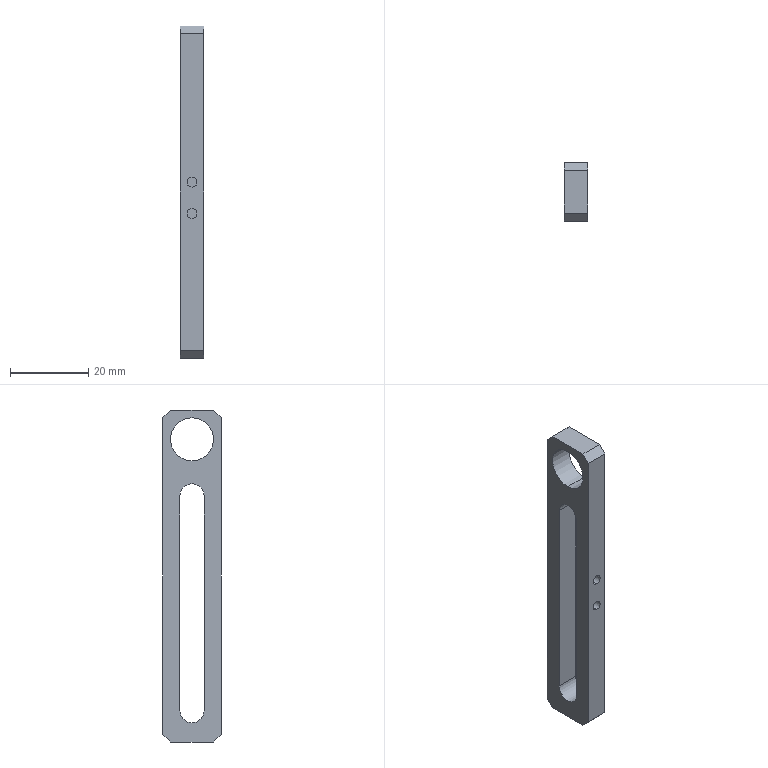Part | SolidWorks | features HoleWzd 2, Chamfer 1, Extrusion 1 | 1 solid | 21 faces | box 6 x 15 x 85 mm | volume 4761 mm3 | plane 12 | cylinder 9 | commonest cylinder face diameters 2.5 x4 6.2 x3 11 x2
STEP:
#1=CARTESIAN_POINT('',(3.,-10.6,-41.25));
#2=VERTEX_POINT('',#1);
#3=CARTESIAN_POINT('',(3.,-10.6,-38.75));
#4=VERTEX_POINT('',#3);
#5=CARTESIAN_POINT('',(3.,-10.6,-40.));
#6=DIRECTION('',(0.,1.,0.));
#7=DIRECTION('',(0.,0.,1.));
#8=AXIS2_PLACEMENT_3D('',#5,#6,#7);
#9=CIRCLE('',#8,1.25);
#10=EDGE_CURVE('',#2,#4,#9,.T.);
#11=ORIENTED_EDGE('',*,*,#10,.T.);
#12=CARTESIAN_POINT('',(3.,-15.,-38.75));
#13=VERTEX_POINT('',#12);
#14=CARTESIAN_POINT('',(3.,-15.,-38.75));
#15=DIRECTION('',(0.,-1.,0.));
#16=VECTOR('',#15,1000.);
#17=LINE('',#14,#16);
#18=EDGE_CURVE('',#4,#13,#17,.T.);
#19=ORIENTED_EDGE('',*,*,#18,.T.);
#20=CARTESIAN_POINT('',(3.,-15.,-41.25));
#21=VERTEX_POINT('',#20);
#22=CARTESIAN_POINT('',(3.,-15.,-40.));
#23=DIRECTION('',(0.,-1.,0.));
#24=DIRECTION('',(0.,0.,-1.));
#25=AXIS2_PLACEMENT_3D('',#22,#23,#24);
#26=CIRCLE('',#25,1.25);
#27=EDGE_CURVE('',#13,#21,#26,.T.);
#28=ORIENTED_EDGE('',*,*,#27,.T.);
#29=CARTESIAN_POINT('',(3.,-15.,-41.25));
#30=DIRECTION('',(0.,-1.,0.));
#31=VECTOR('',#30,1000.);
#32=LINE('',#29,#31);
#33=EDGE_CURVE('',#2,#21,#32,.T.);
#34=ORIENTED_EDGE('',*,*,#33,.F.);
#35=EDGE_LOOP('',(#11,#19,#28,#34));
#36=FACE_OUTER_BOUND('',#35,.T.);
#37=CARTESIAN_POINT('',(3.,-15.,-40.));
#38=DIRECTION('',(0.,-1.,0.));
#39=DIRECTION('',(0.,0.,-1.));
#40=AXIS2_PLACEMENT_3D('',#37,#38,#39);
#41=CYLINDRICAL_SURFACE('',#40,1.25);
#42=ADVANCED_FACE('',(#36),#41,.F.);
#43=CARTESIAN_POINT('',(3.,-10.6,-49.25));
#44=VERTEX_POINT('',#43);
#45=CARTESIAN_POINT('',(3.,-10.6,-46.75));
#46=VERTEX_POINT('',#45);
#47=CARTESIAN_POINT('',(3.,-10.6,-48.));
#48=DIRECTION('',(0.,1.,0.));
#49=DIRECTION('',(0.,0.,1.));
#50=AXIS2_PLACEMENT_3D('',#47,#48,#49);
#51=CIRCLE('',#50,1.25);
#52=EDGE_CURVE('',#44,#46,#51,.T.);
#53=ORIENTED_EDGE('',*,*,#52,.T.);
#54=CARTESIAN_POINT('',(3.,-15.,-46.75));
#55=VERTEX_POINT('',#54);
#56=CARTESIAN_POINT('',(3.,-15.,-46.75));
#57=DIRECTION('',(0.,-1.,0.));
#58=VECTOR('',#57,1000.);
#59=LINE('',#56,#58);
#60=EDGE_CURVE('',#46,#55,#59,.T.);
#61=ORIENTED_EDGE('',*,*,#60,.T.);
#62=CARTESIAN_POINT('',(3.,-15.,-49.25));
#63=VERTEX_POINT('',#62);
#64=CARTESIAN_POINT('',(3.,-15.,-48.));
#65=DIRECTION('',(0.,-1.,0.));
#66=DIRECTION('',(0.,0.,-1.));
#67=AXIS2_PLACEMENT_3D('',#64,#65,#66);
#68=CIRCLE('',#67,1.25);
#69=EDGE_CURVE('',#55,#63,#68,.T.);
#70=ORIENTED_EDGE('',*,*,#69,.T.);
#71=CARTESIAN_POINT('',(3.,-15.,-49.25));
#72=DIRECTION('',(0.,-1.,0.));
#73=VECTOR('',#72,1000.);
#74=LINE('',#71,#73);
#75=EDGE_CURVE('',#44,#63,#74,.T.);
#76=ORIENTED_EDGE('',*,*,#75,.F.);
#77=EDGE_LOOP('',(#53,#61,#70,#76));
#78=FACE_OUTER_BOUND('',#77,.T.);
#79=CARTESIAN_POINT('',(3.,-15.,-48.));
#80=DIRECTION('',(0.,-1.,0.));
#81=DIRECTION('',(0.,0.,-1.));
#82=AXIS2_PLACEMENT_3D('',#79,#80,#81);
#83=CYLINDRICAL_SURFACE('',#82,1.25);
#84=ADVANCED_FACE('',(#78),#83,.F.);
#85=CARTESIAN_POINT('',(0.,-7.5,-2.));
#86=VERTEX_POINT('',#85);
#87=CARTESIAN_POINT('',(0.,-7.5,-13.));
#88=VERTEX_POINT('',#87);
#89=CARTESIAN_POINT('',(0.,-7.5,-7.5));
#90=DIRECTION('',(1.,0.,0.));
#91=DIRECTION('',(0.,0.,-1.));
#92=AXIS2_PLACEMENT_3D('',#89,#90,#91);
#93=CIRCLE('',#92,5.5);
#94=EDGE_CURVE('',#86,#88,#93,.T.);
#95=ORIENTED_EDGE('',*,*,#94,.F.);
#96=CARTESIAN_POINT('',(6.,-7.5,-2.));
#97=VERTEX_POINT('',#96);
#98=CARTESIAN_POINT('',(6.,-7.5,-2.));
#99=DIRECTION('',(1.,0.,0.));
#100=VECTOR('',#99,1000.);
#101=LINE('',#98,#100);
#102=EDGE_CURVE('',#86,#97,#101,.T.);
#103=ORIENTED_EDGE('',*,*,#102,.T.);
#104=CARTESIAN_POINT('',(6.,-7.5,-13.));
#105=VERTEX_POINT('',#104);
#106=CARTESIAN_POINT('',(6.,-7.5,-7.5));
#107=DIRECTION('',(1.,0.,0.));
#108=DIRECTION('',(0.,0.,-1.));
#109=AXIS2_PLACEMENT_3D('',#106,#107,#108);
#110=CIRCLE('',#109,5.5);
#111=EDGE_CURVE('',#97,#105,#110,.T.);
#112=ORIENTED_EDGE('',*,*,#111,.T.);
#113=CARTESIAN_POINT('',(6.,-7.5,-13.));
#114=DIRECTION('',(1.,0.,0.));
#115=VECTOR('',#114,1000.);
#116=LINE('',#113,#115);
#117=EDGE_CURVE('',#88,#105,#116,.T.);
#118=ORIENTED_EDGE('',*,*,#117,.F.);
#119=EDGE_LOOP('',(#95,#103,#112,#118));
#120=FACE_OUTER_BOUND('',#119,.T.);
#121=CARTESIAN_POINT('',(6.,-7.5,-7.5));
#122=DIRECTION('',(1.,0.,0.));
#123=DIRECTION('',(0.,0.,-1.));
#124=AXIS2_PLACEMENT_3D('',#121,#122,#123);
#125=CYLINDRICAL_SURFACE('',#124,5.5);
#126=ADVANCED_FACE('',(#120),#125,.F.);
#127=CARTESIAN_POINT('',(6.,-4.4,-22.));
#128=VERTEX_POINT('',#127);
#129=CARTESIAN_POINT('',(6.,-7.5,-18.9));
#130=VERTEX_POINT('',#129);
#131=CARTESIAN_POINT('',(6.,-7.5,-22.));
#132=DIRECTION('',(1.,0.,0.));
#133=DIRECTION('',(0.,0.,-1.));
#134=AXIS2_PLACEMENT_3D('',#131,#132,#133);
#135=CIRCLE('',#134,3.1);
#136=EDGE_CURVE('',#128,#130,#135,.T.);
#137=ORIENTED_EDGE('',*,*,#136,.T.);
#138=CARTESIAN_POINT('',(0.,-7.5,-18.9));
#139=VERTEX_POINT('',#138);
#140=CARTESIAN_POINT('',(6.,-7.5,-18.9));
#141=DIRECTION('',(-1.,0.,0.));
#142=VECTOR('',#141,1000.);
#143=LINE('',#140,#142);
#144=EDGE_CURVE('',#130,#139,#143,.T.);
#145=ORIENTED_EDGE('',*,*,#144,.T.);
#146=CARTESIAN_POINT('',(0.,-4.4,-22.));
#147=VERTEX_POINT('',#146);
#148=CARTESIAN_POINT('',(0.,-7.5,-22.));
#149=DIRECTION('',(1.,0.,0.));
#150=DIRECTION('',(0.,0.,-1.));
#151=AXIS2_PLACEMENT_3D('',#148,#149,#150);
#152=CIRCLE('',#151,3.1);
#153=EDGE_CURVE('',#147,#139,#152,.T.);
#154=ORIENTED_EDGE('',*,*,#153,.F.);
#155=CARTESIAN_POINT('',(6.,-4.4,-22.));
#156=DIRECTION('',(-1.,0.,0.));
#157=VECTOR('',#156,1000.);
#158=LINE('',#155,#157);
#159=EDGE_CURVE('',#128,#147,#158,.T.);
#160=ORIENTED_EDGE('',*,*,#159,.F.);
#161=EDGE_LOOP('',(#137,#145,#154,#160));
#162=FACE_OUTER_BOUND('',#161,.T.);
#163=CARTESIAN_POINT('',(6.,-7.5,-22.));
#164=DIRECTION('',(-1.,0.,0.));
#165=DIRECTION('',(0.,0.,1.));
#166=AXIS2_PLACEMENT_3D('',#163,#164,#165);
#167=CYLINDRICAL_SURFACE('',#166,3.1);
#168=ADVANCED_FACE('',(#162),#167,.F.);
#169=CARTESIAN_POINT('',(6.,-7.5,-7.5));
#170=DIRECTION('',(1.,0.,0.));
#171=DIRECTION('',(0.,0.,-1.));
#172=AXIS2_PLACEMENT_3D('',#169,#170,#171);
#173=CIRCLE('',#172,5.5);
#174=EDGE_CURVE('',#105,#97,#173,.T.);
#175=ORIENTED_EDGE('',*,*,#174,.F.);
#176=ORIENTED_EDGE('',*,*,#111,.F.);
#177=EDGE_LOOP('',(#175,#176));
#178=FACE_BOUND('',#177,.T.);
#179=CARTESIAN_POINT('',(6.,-13.,-85.));
#180=VERTEX_POINT('',#179);
#181=CARTESIAN_POINT('',(6.,-2.,-85.));
#182=VERTEX_POINT('',#181);
#183=CARTESIAN_POINT('',(6.,0.,-85.));
#184=DIRECTION('',(0.,1.,0.));
#185=VECTOR('',#184,1000.);
#186=LINE('',#183,#185);
#187=EDGE_CURVE('',#180,#182,#186,.T.);
#188=ORIENTED_EDGE('',*,*,#187,.T.);
#189=CARTESIAN_POINT('',(6.,0.,-83.));
#190=VERTEX_POINT('',#189);
#191=CARTESIAN_POINT('',(6.,34.,-49.));
#192=DIRECTION('',(0.,0.7071,0.7071));
#193=VECTOR('',#192,1000.);
#194=LINE('',#191,#193);
#195=EDGE_CURVE('',#182,#190,#194,.T.);
#196=ORIENTED_EDGE('',*,*,#195,.T.);
#197=CARTESIAN_POINT('',(6.,0.,-2.));
#198=VERTEX_POINT('',#197);
#199=CARTESIAN_POINT('',(6.,0.,0.));
#200=DIRECTION('',(0.,0.,1.));
#201=VECTOR('',#200,1000.);
#202=LINE('',#199,#201);
#203=EDGE_CURVE('',#190,#198,#202,.T.);
#204=ORIENTED_EDGE('',*,*,#203,.T.);
#205=CARTESIAN_POINT('',(6.,-2.,0.));
#206=VERTEX_POINT('',#205);
#207=CARTESIAN_POINT('',(6.,-8.5,6.5));
#208=DIRECTION('',(0.,-0.7071,0.7071));
#209=VECTOR('',#208,1000.);
#210=LINE('',#207,#209);
#211=EDGE_CURVE('',#198,#206,#210,.T.);
#212=ORIENTED_EDGE('',*,*,#211,.T.);
#213=CARTESIAN_POINT('',(6.,-13.,0.));
#214=VERTEX_POINT('',#213);
#215=CARTESIAN_POINT('',(6.,0.,0.));
#216=DIRECTION('',(0.,-1.,0.));
#217=VECTOR('',#216,1000.);
#218=LINE('',#215,#217);
#219=EDGE_CURVE('',#206,#214,#218,.T.);
#220=ORIENTED_EDGE('',*,*,#219,.T.);
#221=CARTESIAN_POINT('',(6.,-15.,-2.));
#222=VERTEX_POINT('',#221);
#223=CARTESIAN_POINT('',(6.,-14.,-1.));
#224=DIRECTION('',(0.,-0.7071,-0.7071));
#225=VECTOR('',#224,1000.);
#226=LINE('',#223,#225);
#227=EDGE_CURVE('',#214,#222,#226,.T.);
#228=ORIENTED_EDGE('',*,*,#227,.T.);
#229=CARTESIAN_POINT('',(6.,-15.,-83.));
#230=VERTEX_POINT('',#229);
#231=CARTESIAN_POINT('',(6.,-15.,0.));
#232=DIRECTION('',(0.,0.,-1.));
#233=VECTOR('',#232,1000.);
#234=LINE('',#231,#233);
#235=EDGE_CURVE('',#222,#230,#234,.T.);
#236=ORIENTED_EDGE('',*,*,#235,.T.);
#237=CARTESIAN_POINT('',(6.,-56.5,-41.5));
#238=DIRECTION('',(0.,0.7071,-0.7071));
#239=VECTOR('',#238,1000.);
#240=LINE('',#237,#239);
#241=EDGE_CURVE('',#230,#180,#240,.T.);
#242=ORIENTED_EDGE('',*,*,#241,.T.);
#243=EDGE_LOOP('',(#188,#196,#204,#212,#220,#228,#236,#242));
#244=FACE_OUTER_BOUND('',#243,.T.);
#245=CARTESIAN_POINT('',(6.,-10.6,-22.));
#246=VERTEX_POINT('',#245);
#247=CARTESIAN_POINT('',(6.,-10.6,-77.));
#248=VERTEX_POINT('',#247);
#249=CARTESIAN_POINT('',(6.,-10.6,-22.));
#250=DIRECTION('',(0.,0.,-1.));
#251=VECTOR('',#250,1000.);
#252=LINE('',#249,#251);
#253=EDGE_CURVE('',#246,#248,#252,.T.);
#254=ORIENTED_EDGE('',*,*,#253,.F.);
#255=CARTESIAN_POINT('',(6.,-7.5,-22.));
#256=DIRECTION('',(1.,0.,0.));
#257=DIRECTION('',(0.,0.,-1.));
#258=AXIS2_PLACEMENT_3D('',#255,#256,#257);
#259=CIRCLE('',#258,3.1);
#260=EDGE_CURVE('',#130,#246,#259,.T.);
#261=ORIENTED_EDGE('',*,*,#260,.F.);
#262=ORIENTED_EDGE('',*,*,#136,.F.);
#263=CARTESIAN_POINT('',(6.,-4.4,-77.));
#264=VERTEX_POINT('',#263);
#265=CARTESIAN_POINT('',(6.,-4.4,-22.));
#266=DIRECTION('',(0.,0.,1.));
#267=VECTOR('',#266,1000.);
#268=LINE('',#265,#267);
#269=EDGE_CURVE('',#264,#128,#268,.T.);
#270=ORIENTED_EDGE('',*,*,#269,.F.);
#271=CARTESIAN_POINT('',(6.,-7.5,-77.));
#272=DIRECTION('',(1.,0.,0.));
#273=DIRECTION('',(0.,0.,-1.));
#274=AXIS2_PLACEMENT_3D('',#271,#272,#273);
#275=CIRCLE('',#274,3.1);
#276=EDGE_CURVE('',#248,#264,#275,.T.);
#277=ORIENTED_EDGE('',*,*,#276,.F.);
#278=EDGE_LOOP('',(#254,#261,#262,#270,#277));
#279=FACE_BOUND('',#278,.T.);
#280=CARTESIAN_POINT('',(6.,-15.,0.));
#281=DIRECTION('',(1.,0.,0.));
#282=DIRECTION('',(0.,0.,-1.));
#283=AXIS2_PLACEMENT_3D('',#280,#281,#282);
#284=PLANE('',#283);
#285=ADVANCED_FACE('',(#178,#244,#279),#284,.T.);
#286=CARTESIAN_POINT('',(0.,-7.5,-7.5));
#287=DIRECTION('',(1.,0.,0.));
#288=DIRECTION('',(0.,0.,-1.));
#289=AXIS2_PLACEMENT_3D('',#286,#287,#288);
#290=CIRCLE('',#289,5.5);
#291=EDGE_CURVE('',#88,#86,#290,.T.);
#292=ORIENTED_EDGE('',*,*,#291,.T.);
#293=ORIENTED_EDGE('',*,*,#94,.T.);
#294=EDGE_LOOP('',(#292,#293));
#295=FACE_BOUND('',#294,.T.);
#296=CARTESIAN_POINT('',(0.,0.,-83.));
#297=VERTEX_POINT('',#296);
#298=CARTESIAN_POINT('',(0.,0.,-2.));
#299=VERTEX_POINT('',#298);
#300=CARTESIAN_POINT('',(0.,0.,0.));
#301=DIRECTION('',(0.,0.,1.));
#302=VECTOR('',#301,1000.);
#303=LINE('',#300,#302);
#304=EDGE_CURVE('',#297,#299,#303,.T.);
#305=ORIENTED_EDGE('',*,*,#304,.F.);
#306=CARTESIAN_POINT('',(0.,-2.,-85.));
#307=VERTEX_POINT('',#306);
#308=CARTESIAN_POINT('',(0.,0.,-83.));
#309=DIRECTION('',(0.,-0.7071,-0.7071));
#310=VECTOR('',#309,1000.);
#311=LINE('',#308,#310);
#312=EDGE_CURVE('',#297,#307,#311,.T.);
#313=ORIENTED_EDGE('',*,*,#312,.T.);
#314=CARTESIAN_POINT('',(0.,-13.,-85.));
#315=VERTEX_POINT('',#314);
#316=CARTESIAN_POINT('',(0.,0.,-85.));
#317=DIRECTION('',(0.,1.,0.));
#318=VECTOR('',#317,1000.);
#319=LINE('',#316,#318);
#320=EDGE_CURVE('',#315,#307,#319,.T.);
#321=ORIENTED_EDGE('',*,*,#320,.F.);
#322=CARTESIAN_POINT('',(0.,-15.,-83.));
#323=VERTEX_POINT('',#322);
#324=CARTESIAN_POINT('',(0.,-13.,-85.));
#325=DIRECTION('',(0.,-0.7071,0.7071));
#326=VECTOR('',#325,1000.);
#327=LINE('',#324,#326);
#328=EDGE_CURVE('',#315,#323,#327,.T.);
#329=ORIENTED_EDGE('',*,*,#328,.T.);
#330=CARTESIAN_POINT('',(0.,-15.,-2.));
#331=VERTEX_POINT('',#330);
#332=CARTESIAN_POINT('',(0.,-15.,0.));
#333=DIRECTION('',(0.,0.,-1.));
#334=VECTOR('',#333,1000.);
#335=LINE('',#332,#334);
#336=EDGE_CURVE('',#331,#323,#335,.T.);
#337=ORIENTED_EDGE('',*,*,#336,.F.);
#338=CARTESIAN_POINT('',(0.,-13.,0.));
#339=VERTEX_POINT('',#338);
#340=CARTESIAN_POINT('',(0.,-15.,-2.));
#341=DIRECTION('',(0.,0.7071,0.7071));
#342=VECTOR('',#341,1000.);
#343=LINE('',#340,#342);
#344=EDGE_CURVE('',#331,#339,#343,.T.);
#345=ORIENTED_EDGE('',*,*,#344,.T.);
#346=CARTESIAN_POINT('',(0.,-2.,0.));
#347=VERTEX_POINT('',#346);
#348=CARTESIAN_POINT('',(0.,0.,0.));
#349=DIRECTION('',(0.,-1.,0.));
#350=VECTOR('',#349,1000.);
#351=LINE('',#348,#350);
#352=EDGE_CURVE('',#347,#339,#351,.T.);
#353=ORIENTED_EDGE('',*,*,#352,.F.);
#354=CARTESIAN_POINT('',(0.,-2.,0.));
#355=DIRECTION('',(0.,0.7071,-0.7071));
#356=VECTOR('',#355,1000.);
#357=LINE('',#354,#356);
#358=EDGE_CURVE('',#347,#299,#357,.T.);
#359=ORIENTED_EDGE('',*,*,#358,.T.);
#360=EDGE_LOOP('',(#305,#313,#321,#329,#337,#345,#353,#359));
#361=FACE_OUTER_BOUND('',#360,.T.);
#362=ORIENTED_EDGE('',*,*,#153,.T.);
#363=CARTESIAN_POINT('',(0.,-10.6,-22.));
#364=VERTEX_POINT('',#363);
#365=CARTESIAN_POINT('',(0.,-7.5,-22.));
#366=DIRECTION('',(1.,0.,0.));
#367=DIRECTION('',(0.,0.,-1.));
#368=AXIS2_PLACEMENT_3D('',#365,#366,#367);
#369=CIRCLE('',#368,3.1);
#370=EDGE_CURVE('',#139,#364,#369,.T.);
#371=ORIENTED_EDGE('',*,*,#370,.T.);
#372=CARTESIAN_POINT('',(0.,-10.6,-77.));
#373=VERTEX_POINT('',#372);
#374=CARTESIAN_POINT('',(0.,-10.6,-22.));
#375=DIRECTION('',(0.,0.,-1.));
#376=VECTOR('',#375,1000.);
#377=LINE('',#374,#376);
#378=EDGE_CURVE('',#364,#373,#377,.T.);
#379=ORIENTED_EDGE('',*,*,#378,.T.);
#380=CARTESIAN_POINT('',(0.,-4.4,-77.));
#381=VERTEX_POINT('',#380);
#382=CARTESIAN_POINT('',(0.,-7.5,-77.));
#383=DIRECTION('',(1.,0.,0.));
#384=DIRECTION('',(0.,0.,-1.));
#385=AXIS2_PLACEMENT_3D('',#382,#383,#384);
#386=CIRCLE('',#385,3.1);
#387=EDGE_CURVE('',#373,#381,#386,.T.);
#388=ORIENTED_EDGE('',*,*,#387,.T.);
#389=CARTESIAN_POINT('',(0.,-4.4,-22.));
#390=DIRECTION('',(0.,0.,1.));
#391=VECTOR('',#390,1000.);
#392=LINE('',#389,#391);
#393=EDGE_CURVE('',#381,#147,#392,.T.);
#394=ORIENTED_EDGE('',*,*,#393,.T.);
#395=EDGE_LOOP('',(#362,#371,#379,#388,#394));
#396=FACE_BOUND('',#395,.T.);
#397=CARTESIAN_POINT('',(0.,-15.,0.));
#398=DIRECTION('',(1.,0.,0.));
#399=DIRECTION('',(0.,0.,-1.));
#400=AXIS2_PLACEMENT_3D('',#397,#398,#399);
#401=PLANE('',#400);
#402=ADVANCED_FACE('',(#295,#361,#396),#401,.F.);
#403=ORIENTED_EDGE('',*,*,#352,.T.);
#404=CARTESIAN_POINT('',(6.,-13.,0.));
#405=DIRECTION('',(1.,0.,0.));
#406=VECTOR('',#405,1000.);
#407=LINE('',#404,#406);
#408=EDGE_CURVE('',#339,#214,#407,.T.);
#409=ORIENTED_EDGE('',*,*,#408,.T.);
#410=ORIENTED_EDGE('',*,*,#219,.F.);
#411=CARTESIAN_POINT('',(6.,-2.,0.));
#412=DIRECTION('',(-1.,0.,0.));
#413=VECTOR('',#412,1000.);
#414=LINE('',#411,#413);
#415=EDGE_CURVE('',#206,#347,#414,.T.);
#416=ORIENTED_EDGE('',*,*,#415,.T.);
#417=EDGE_LOOP('',(#403,#409,#410,#416));
#418=FACE_OUTER_BOUND('',#417,.T.);
#419=CARTESIAN_POINT('',(6.,0.,0.));
#420=DIRECTION('',(0.,0.,-1.));
#421=DIRECTION('',(0.,1.,0.));
#422=AXIS2_PLACEMENT_3D('',#419,#420,#421);
#423=PLANE('',#422);
#424=ADVANCED_FACE('',(#418),#423,.F.);
#425=CARTESIAN_POINT('',(3.,-15.,-40.));
#426=DIRECTION('',(0.,-1.,0.));
#427=DIRECTION('',(0.,0.,-1.));
#428=AXIS2_PLACEMENT_3D('',#425,#426,#427);
#429=CIRCLE('',#428,1.25);
#430=EDGE_CURVE('',#21,#13,#429,.T.);
#431=ORIENTED_EDGE('',*,*,#430,.F.);
#432=ORIENTED_EDGE('',*,*,#27,.F.);
#433=EDGE_LOOP('',(#431,#432));
#434=FACE_BOUND('',#433,.T.);
#435=CARTESIAN_POINT('',(3.,-15.,-48.));
#436=DIRECTION('',(0.,-1.,0.));
#437=DIRECTION('',(0.,0.,-1.));
#438=AXIS2_PLACEMENT_3D('',#435,#436,#437);
#439=CIRCLE('',#438,1.25);
#440=EDGE_CURVE('',#63,#55,#439,.T.);
#441=ORIENTED_EDGE('',*,*,#440,.F.);
#442=ORIENTED_EDGE('',*,*,#69,.F.);
#443=EDGE_LOOP('',(#441,#442));
#444=FACE_BOUND('',#443,.T.);
#445=ORIENTED_EDGE('',*,*,#336,.T.);
#446=CARTESIAN_POINT('',(6.,-15.,-83.));
#447=DIRECTION('',(1.,0.,0.));
#448=VECTOR('',#447,1000.);
#449=LINE('',#446,#448);
#450=EDGE_CURVE('',#323,#230,#449,.T.);
#451=ORIENTED_EDGE('',*,*,#450,.T.);
#452=ORIENTED_EDGE('',*,*,#235,.F.);
#453=CARTESIAN_POINT('',(6.,-15.,-2.));
#454=DIRECTION('',(-1.,0.,0.));
#455=VECTOR('',#454,1000.);
#456=LINE('',#453,#455);
#457=EDGE_CURVE('',#222,#331,#456,.T.);
#458=ORIENTED_EDGE('',*,*,#457,.T.);
#459=EDGE_LOOP('',(#445,#451,#452,#458));
#460=FACE_OUTER_BOUND('',#459,.T.);
#461=CARTESIAN_POINT('',(6.,-15.,0.));
#462=DIRECTION('',(0.,1.,0.));
#463=DIRECTION('',(0.,0.,1.));
#464=AXIS2_PLACEMENT_3D('',#461,#462,#463);
#465=PLANE('',#464);
#466=ADVANCED_FACE('',(#434,#444,#460),#465,.F.);
#467=ORIENTED_EDGE('',*,*,#320,.T.);
#468=CARTESIAN_POINT('',(6.,-2.,-85.));
#469=DIRECTION('',(1.,0.,0.));
#470=VECTOR('',#469,1000.);
#471=LINE('',#468,#470);
#472=EDGE_CURVE('',#307,#182,#471,.T.);
#473=ORIENTED_EDGE('',*,*,#472,.T.);
#474=ORIENTED_EDGE('',*,*,#187,.F.);
#475=CARTESIAN_POINT('',(6.,-13.,-85.));
#476=DIRECTION('',(-1.,0.,0.));
#477=VECTOR('',#476,1000.);
#478=LINE('',#475,#477);
#479=EDGE_CURVE('',#180,#315,#478,.T.);
#480=ORIENTED_EDGE('',*,*,#479,.T.);
#481=EDGE_LOOP('',(#467,#473,#474,#480));
#482=FACE_OUTER_BOUND('',#481,.T.);
#483=CARTESIAN_POINT('',(6.,0.,-85.));
#484=DIRECTION('',(0.,0.,1.));
#485=DIRECTION('',(1.,0.,0.));
#486=AXIS2_PLACEMENT_3D('',#483,#484,#485);
#487=PLANE('',#486);
#488=ADVANCED_FACE('',(#482),#487,.F.);
#489=ORIENTED_EDGE('',*,*,#203,.F.);
#490=CARTESIAN_POINT('',(6.,0.,-83.));
#491=DIRECTION('',(-1.,0.,0.));
#492=VECTOR('',#491,1000.);
#493=LINE('',#490,#492);
#494=EDGE_CURVE('',#190,#297,#493,.T.);
#495=ORIENTED_EDGE('',*,*,#494,.T.);
#496=ORIENTED_EDGE('',*,*,#304,.T.);
#497=CARTESIAN_POINT('',(6.,0.,-2.));
#498=DIRECTION('',(1.,0.,0.));
#499=VECTOR('',#498,1000.);
#500=LINE('',#497,#499);
#501=EDGE_CURVE('',#299,#198,#500,.T.);
#502=ORIENTED_EDGE('',*,*,#501,.T.);
#503=EDGE_LOOP('',(#489,#495,#496,#502));
#504=FACE_OUTER_BOUND('',#503,.T.);
#505=CARTESIAN_POINT('',(6.,0.,0.));
#506=DIRECTION('',(0.,-1.,0.));
#507=DIRECTION('',(0.,0.,-1.));
#508=AXIS2_PLACEMENT_3D('',#505,#506,#507);
#509=PLANE('',#508);
#510=ADVANCED_FACE('',(#504),#509,.F.);
#511=ORIENTED_EDGE('',*,*,#144,.F.);
#512=ORIENTED_EDGE('',*,*,#260,.T.);
#513=CARTESIAN_POINT('',(6.,-10.6,-22.));
#514=DIRECTION('',(-1.,0.,0.));
#515=VECTOR('',#514,1000.);
#516=LINE('',#513,#515);
#517=EDGE_CURVE('',#246,#364,#516,.T.);
#518=ORIENTED_EDGE('',*,*,#517,.T.);
#519=ORIENTED_EDGE('',*,*,#370,.F.);
#520=EDGE_LOOP('',(#511,#512,#518,#519));
#521=FACE_OUTER_BOUND('',#520,.T.);
#522=CARTESIAN_POINT('',(6.,-7.5,-22.));
#523=DIRECTION('',(-1.,0.,0.));
#524=DIRECTION('',(0.,0.,1.));
#525=AXIS2_PLACEMENT_3D('',#522,#523,#524);
#526=CYLINDRICAL_SURFACE('',#525,3.1);
#527=ADVANCED_FACE('',(#521),#526,.F.);
#528=ORIENTED_EDGE('',*,*,#10,.F.);
#529=CARTESIAN_POINT('',(3.,-10.6,-40.));
#530=DIRECTION('',(0.,1.,0.));
#531=DIRECTION('',(0.,0.,1.));
#532=AXIS2_PLACEMENT_3D('',#529,#530,#531);
#533=CIRCLE('',#532,1.25);
#534=EDGE_CURVE('',#4,#2,#533,.T.);
#535=ORIENTED_EDGE('',*,*,#534,.F.);
#536=EDGE_LOOP('',(#528,#535));
#537=FACE_BOUND('',#536,.T.);
#538=ORIENTED_EDGE('',*,*,#52,.F.);
#539=CARTESIAN_POINT('',(3.,-10.6,-48.));
#540=DIRECTION('',(0.,1.,0.));
#541=DIRECTION('',(0.,0.,1.));
#542=AXIS2_PLACEMENT_3D('',#539,#540,#541);
#543=CIRCLE('',#542,1.25);
#544=EDGE_CURVE('',#46,#44,#543,.T.);
#545=ORIENTED_EDGE('',*,*,#544,.F.);
#546=EDGE_LOOP('',(#538,#545));
#547=FACE_BOUND('',#546,.T.);
#548=ORIENTED_EDGE('',*,*,#378,.F.);
#549=ORIENTED_EDGE('',*,*,#517,.F.);
#550=ORIENTED_EDGE('',*,*,#253,.T.);
#551=CARTESIAN_POINT('',(6.,-10.6,-77.));
#552=DIRECTION('',(-1.,0.,0.));
#553=VECTOR('',#552,1000.);
#554=LINE('',#551,#553);
#555=EDGE_CURVE('',#248,#373,#554,.T.);
#556=ORIENTED_EDGE('',*,*,#555,.T.);
#557=EDGE_LOOP('',(#548,#549,#550,#556));
#558=FACE_OUTER_BOUND('',#557,.T.);
#559=CARTESIAN_POINT('',(6.,-10.6,-22.));
#560=DIRECTION('',(0.,1.,0.));
#561=DIRECTION('',(0.,0.,1.));
#562=AXIS2_PLACEMENT_3D('',#559,#560,#561);
#563=PLANE('',#562);
#564=ADVANCED_FACE('',(#537,#547,#558),#563,.T.);
#565=ORIENTED_EDGE('',*,*,#387,.F.);
#566=ORIENTED_EDGE('',*,*,#555,.F.);
#567=ORIENTED_EDGE('',*,*,#276,.T.);
#568=CARTESIAN_POINT('',(6.,-4.4,-77.));
#569=DIRECTION('',(-1.,0.,0.));
#570=VECTOR('',#569,1000.);
#571=LINE('',#568,#570);
#572=EDGE_CURVE('',#264,#381,#571,.T.);
#573=ORIENTED_EDGE('',*,*,#572,.T.);
#574=EDGE_LOOP('',(#565,#566,#567,#573));
#575=FACE_OUTER_BOUND('',#574,.T.);
#576=CARTESIAN_POINT('',(6.,-7.5,-77.));
#577=DIRECTION('',(-1.,0.,0.));
#578=DIRECTION('',(0.,0.,1.));
#579=AXIS2_PLACEMENT_3D('',#576,#577,#578);
#580=CYLINDRICAL_SURFACE('',#579,3.1);
#581=ADVANCED_FACE('',(#575),#580,.F.);
#582=ORIENTED_EDGE('',*,*,#393,.F.);
#583=ORIENTED_EDGE('',*,*,#572,.F.);
#584=ORIENTED_EDGE('',*,*,#269,.T.);
#585=ORIENTED_EDGE('',*,*,#159,.T.);
#586=EDGE_LOOP('',(#582,#583,#584,#585));
#587=FACE_OUTER_BOUND('',#586,.T.);
#588=CARTESIAN_POINT('',(6.,-4.4,-22.));
#589=DIRECTION('',(0.,-1.,0.));
#590=DIRECTION('',(0.,0.,-1.));
#591=AXIS2_PLACEMENT_3D('',#588,#589,#590);
#592=PLANE('',#591);
#593=ADVANCED_FACE('',(#587),#592,.T.);
#594=ORIENTED_EDGE('',*,*,#102,.F.);
#595=ORIENTED_EDGE('',*,*,#291,.F.);
#596=ORIENTED_EDGE('',*,*,#117,.T.);
#597=ORIENTED_EDGE('',*,*,#174,.T.);
#598=EDGE_LOOP('',(#594,#595,#596,#597));
#599=FACE_OUTER_BOUND('',#598,.T.);
#600=CARTESIAN_POINT('',(6.,-7.5,-7.5));
#601=DIRECTION('',(1.,0.,0.));
#602=DIRECTION('',(0.,0.,-1.));
#603=AXIS2_PLACEMENT_3D('',#600,#601,#602);
#604=CYLINDRICAL_SURFACE('',#603,5.5);
#605=ADVANCED_FACE('',(#599),#604,.F.);
#606=ORIENTED_EDGE('',*,*,#195,.F.);
#607=ORIENTED_EDGE('',*,*,#472,.F.);
#608=ORIENTED_EDGE('',*,*,#312,.F.);
#609=ORIENTED_EDGE('',*,*,#494,.F.);
#610=EDGE_LOOP('',(#606,#607,#608,#609));
#611=FACE_OUTER_BOUND('',#610,.T.);
#612=CARTESIAN_POINT('',(6.,0.,-83.));
#613=DIRECTION('',(0.,-0.7071,0.7071));
#614=DIRECTION('',(0.,-0.7071,-0.7071));
#615=AXIS2_PLACEMENT_3D('',#612,#613,#614);
#616=PLANE('',#615);
#617=ADVANCED_FACE('',(#611),#616,.F.);
#618=ORIENTED_EDGE('',*,*,#241,.F.);
#619=ORIENTED_EDGE('',*,*,#450,.F.);
#620=ORIENTED_EDGE('',*,*,#328,.F.);
#621=ORIENTED_EDGE('',*,*,#479,.F.);
#622=EDGE_LOOP('',(#618,#619,#620,#621));
#623=FACE_OUTER_BOUND('',#622,.T.);
#624=CARTESIAN_POINT('',(6.,-13.,-85.));
#625=DIRECTION('',(0.,0.7071,0.7071));
#626=DIRECTION('',(0.,-0.7071,0.7071));
#627=AXIS2_PLACEMENT_3D('',#624,#625,#626);
#628=PLANE('',#627);
#629=ADVANCED_FACE('',(#623),#628,.F.);
#630=ORIENTED_EDGE('',*,*,#227,.F.);
#631=ORIENTED_EDGE('',*,*,#408,.F.);
#632=ORIENTED_EDGE('',*,*,#344,.F.);
#633=ORIENTED_EDGE('',*,*,#457,.F.);
#634=EDGE_LOOP('',(#630,#631,#632,#633));
#635=FACE_OUTER_BOUND('',#634,.T.);
#636=CARTESIAN_POINT('',(6.,-15.,-2.));
#637=DIRECTION('',(0.,0.7071,-0.7071));
#638=DIRECTION('',(0.,0.7071,0.7071));
#639=AXIS2_PLACEMENT_3D('',#636,#637,#638);
#640=PLANE('',#639);
#641=ADVANCED_FACE('',(#635),#640,.F.);
#642=ORIENTED_EDGE('',*,*,#211,.F.);
#643=ORIENTED_EDGE('',*,*,#501,.F.);
#644=ORIENTED_EDGE('',*,*,#358,.F.);
#645=ORIENTED_EDGE('',*,*,#415,.F.);
#646=EDGE_LOOP('',(#642,#643,#644,#645));
#647=FACE_OUTER_BOUND('',#646,.T.);
#648=CARTESIAN_POINT('',(6.,-2.,0.));
#649=DIRECTION('',(0.,-0.7071,-0.7071));
#650=DIRECTION('',(0.,0.7071,-0.7071));
#651=AXIS2_PLACEMENT_3D('',#648,#649,#650);
#652=PLANE('',#651);
#653=ADVANCED_FACE('',(#647),#652,.F.);
#654=ORIENTED_EDGE('',*,*,#60,.F.);
#655=ORIENTED_EDGE('',*,*,#544,.T.);
#656=ORIENTED_EDGE('',*,*,#75,.T.);
#657=ORIENTED_EDGE('',*,*,#440,.T.);
#658=EDGE_LOOP('',(#654,#655,#656,#657));
#659=FACE_OUTER_BOUND('',#658,.T.);
#660=CARTESIAN_POINT('',(3.,-15.,-48.));
#661=DIRECTION('',(0.,-1.,0.));
#662=DIRECTION('',(0.,0.,-1.));
#663=AXIS2_PLACEMENT_3D('',#660,#661,#662);
#664=CYLINDRICAL_SURFACE('',#663,1.25);
#665=ADVANCED_FACE('',(#659),#664,.F.);
#666=ORIENTED_EDGE('',*,*,#18,.F.);
#667=ORIENTED_EDGE('',*,*,#534,.T.);
#668=ORIENTED_EDGE('',*,*,#33,.T.);
#669=ORIENTED_EDGE('',*,*,#430,.T.);
#670=EDGE_LOOP('',(#666,#667,#668,#669));
#671=FACE_OUTER_BOUND('',#670,.T.);
#672=CARTESIAN_POINT('',(3.,-15.,-40.));
#673=DIRECTION('',(0.,-1.,0.));
#674=DIRECTION('',(0.,0.,-1.));
#675=AXIS2_PLACEMENT_3D('',#672,#673,#674);
#676=CYLINDRICAL_SURFACE('',#675,1.25);
#677=ADVANCED_FACE('',(#671),#676,.F.);
#678=CLOSED_SHELL('',(#42,#84,#126,#168,#285,#402,#424,#466,#488,#510,#527,#564,#581,#593,#605,#617,#629,#641,#653,#665,#677));
#679=MANIFOLD_SOLID_BREP('',#678);
#680=CARTESIAN_POINT('',(0.,0.,0.));
#681=DIRECTION('',(0.,0.,1.));
#682=DIRECTION('',(1.,0.,0.));
#683=AXIS2_PLACEMENT_3D('',#680,#681,#682);
#684=(LENGTH_UNIT()NAMED_UNIT(*)SI_UNIT(.MILLI.,.METRE.));
#685=UNCERTAINTY_MEASURE_WITH_UNIT(LENGTH_MEASURE(0.00001),#684,'','');
#686=(NAMED_UNIT(*)PLANE_ANGLE_UNIT()SI_UNIT($,.RADIAN.));
#687=(NAMED_UNIT(*)SI_UNIT($,.STERADIAN.)SOLID_ANGLE_UNIT());
#688=(GEOMETRIC_REPRESENTATION_CONTEXT(3)GLOBAL_UNCERTAINTY_ASSIGNED_CONTEXT((#685))GLOBAL_UNIT_ASSIGNED_CONTEXT((#684,#686,#687))REPRESENTATION_CONTEXT('',''));
#689=ADVANCED_BREP_SHAPE_REPRESENTATION('',(#679,#683),#688);